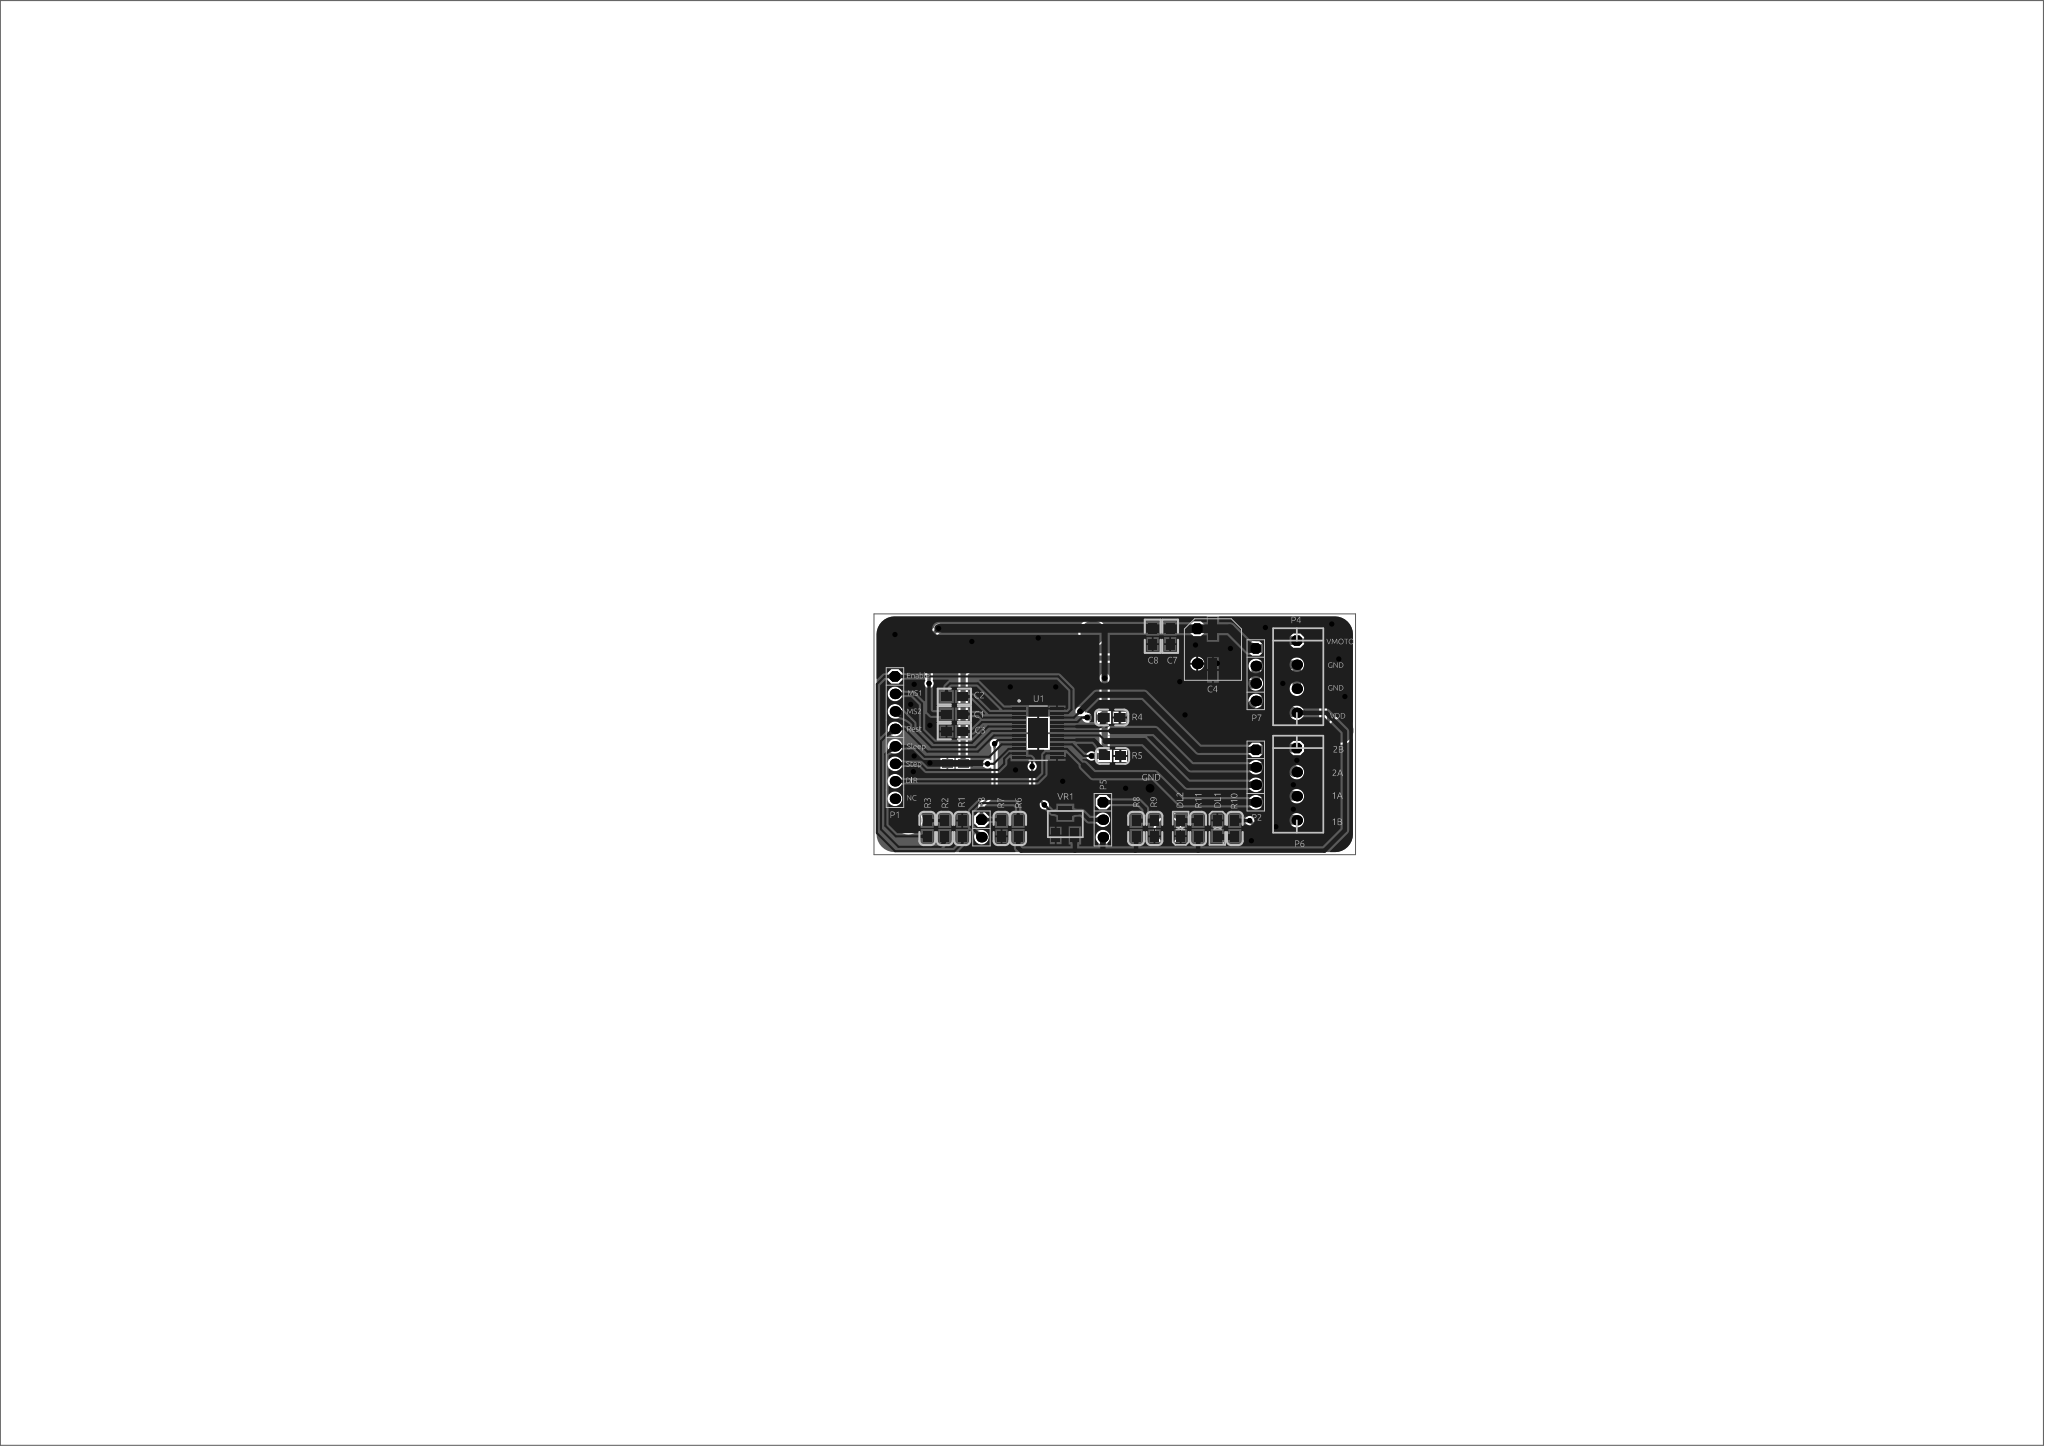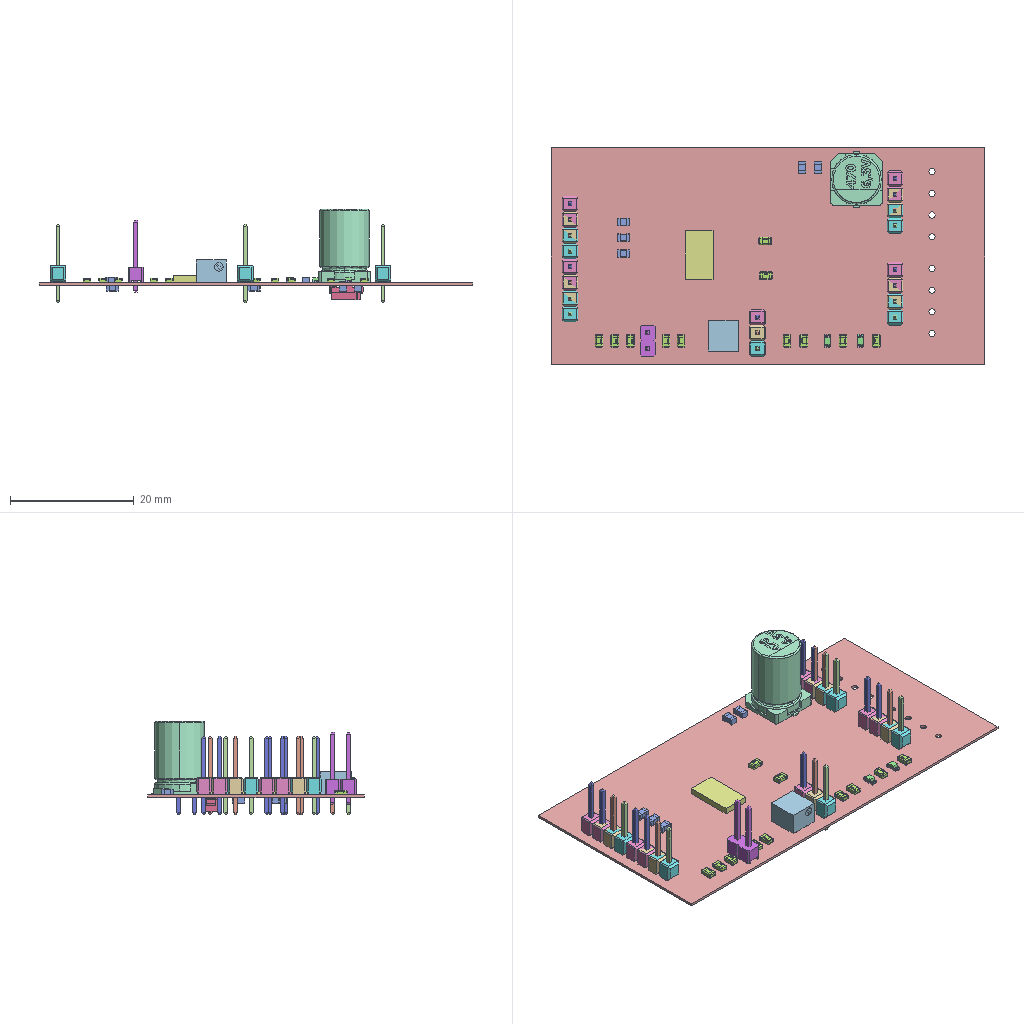Circuit board layout | Altium Designer | box 70 x 35 x 15.1 mm
Layer stack:
# Altium Designer layer stack of  (unit mm; dielectric type: 0 none, 1 core, 2 prepreg, 3 surface material)
index,name,kind,layer,copper_thickness_mm,dielectric_type,dielectric_thickness_mm,dielectric_material,dielectric_constant
0,Top Paste,other,,,,,,
1,Top Overlay,other,,,,,,
2,Top Solder,dielectric,,,3,0.0102,Solder Resist,3.5
3,Top Layer,copper,Top Layer,0.0356,,,,
4,Dielectric 1,dielectric,,,0,0.32,FR-4,4.8
5,Bottom Layer,copper,Bottom Layer,0.0356,,,,
6,Bottom Solder,dielectric,,,3,0.0102,Solder Resist,3.5
7,Bottom Overlay,other,,,,,,
8,Bottom Paste,other,,,,,,
# drill layer pairs: low layer,high layer
drill_pair,Top Layer,Bottom Layer
Part placement:
Designator,Comment,Layer,Footprint,Center-X(mm),Center-Y(mm),Rotation
C10,0.1uF,BottomLayer,0805C,34.671,19.939,360
C11,0.1uF,BottomLayer,0805C,11.811,13.208,180
R11,4.7KΩ,TopLayer,0805R,47.117,3.81,90
R10,2.5KΩ,TopLayer,0805R,52.451,3.81,270
R8,2KΩ,TopLayer,0805R,38.1,3.81,90
R7,0Ω,TopLayer,0805R,18.542,3.81,90
R6,0Ω,TopLayer,0805R,20.955,3.81,270
R5,0.47Ω,TopLayer,0805R,34.671,14.351,180
R4,0.47Ω,TopLayer,0805R,34.544,19.939,180
R3,100KΩ,TopLayer,0805R,7.747,3.81,90
R2,100KΩ,TopLayer,0805R,10.287,3.81,90
R1,10KΩ,TopLayer,0805R,12.827,3.81,90
DL2,COLOR,TopLayer,0805D,44.577,3.837,270
DL1,COLOR,TopLayer,0805D,49.911,3.837,90
C9,0.1uF,BottomLayer,0805C,34.671,14.351,360
C8,0.1uF,TopLayer,0805C,40.513,31.75,270
C7,1uF,TopLayer,0805C,43.053,31.75,270
C6,0.1uF,BottomLayer,0805C,51.435,20.32,270
C5,1uF,BottomLayer,0805C,49.022,20.32,270
C3,0.22uF,TopLayer,0805C,11.684,17.907,180
C2,0.1uF,TopLayer,0805C,11.684,22.987,180
C1,0.1uF,TopLayer,0805C,11.684,20.447,360
D1,1N5822,BottomLayer,1N5822,49.53,24.765,360
R9,3KΩ,TopLayer,0805R,40.767,3.81,270
VR1,10KΩ,TopLayer,3224W,27.813,4.445,0
U1,Value,TopLayer,A4982,23.876,17.653,0
P7,Header(4PIN),TopLayer,排针(4PIN),55.499,26.162,270
P6,VH-3.5-4PIN,TopLayer,VH-3.5-4PIN,61.468,10.244,270
P5,Pin header (3PIN),TopLayer,排针(3PIN),33.274,5.08,270
P3,Header2PIN,TopLayer,排针2PIN,15.621,3.81,270
P2,Header(4PIN),TopLayer,排针(4PIN),55.499,11.43,270
P1,Header(8PIN),TopLayer,排针（8PIN）,3.048,17.018,270
C4,470uF,TopLayer,CAP-SMD_Aluminum_Capacitors_F8_220uF_35V,49.276,29.845,270
P4,VH-3.5-4PIN,TopLayer,VH-3.5-4PIN,61.468,25.865,270
Pad and via stacks:
# Altium Designer via and pad stacks of  (unit mm). Each distinct definition once, with the count of objects using it.
# via: kind,start_layer,end_layer,hole_mm,diameter_mm,mode(0 simple;1 top-mid-bottom;2 full stack),diameter_per_layer,count,example_net
# pad: kind,layer,hole_mm,hole_type(0 round;1 square;2 slot),plating,top_size,top_shape(1 round;2 rect;3 octagon;9 rounded rect),mid_size,bottom_size,mode,footprint,size_per_layer,count,example
pad,Top Layer,0,0,plated,3.2x1.2,2,3.2x1.2,3.2x1.2,0,CAP-SMD Aluminum Capacitors F8 220uF 35V,,2,C4.2
pad,Top Layer,0,0,plated,2x2.032,2,2x2.032,2x2.032,0,3224W,,1,VR1.2
pad,Top Layer,0,0,plated,1.2x2.032,2,1.2x2.032,1.2x2.032,0,3224W,,2,VR1.1
pad,Top Layer,0,0,plated,0.4x2,2,0.4x2,0.4x2,0,A4982,,24,U1.13
pad,Top Layer,0,0,plated,2.85x4.32,2,2.85x4.32,2.85x4.32,0,A4982,,1,U1.24
pad,Top Layer,0,0,plated,1.524x1.27,2,1.524x1.27,1.524x1.27,0,0805R,,22,R9.2
pad,Top Layer,0,0,plated,1.524x1.27,2,1.524x1.27,1.524x1.27,0,0805D,,4,DL2.1
pad,Top Layer,0,0,plated,1.524x1.27,2,1.524x1.27,1.524x1.27,0,0805C,,10,C7.1
pad,Multi-Layer,0.889,0,plated,1.575x1.575,1,1.575x1.575,1.575x1.575,0,,,1,2
pad,Multi-Layer,0.889,0,plated,1.575x1.575,3,1.575x1.575,1.575x1.575,0,,,1,1
pad,Multi-Layer,1,0,plated,1.5x1.5,3,1.5x1.5,1.5x1.5,0,VH-3.5-4PIN,,2,P6.1
pad,Multi-Layer,1,0,plated,1.5x1.5,1,1.5x1.5,1.5x1.5,0,VH-3.5-4PIN,,6,P6.2
pad,Multi-Layer,0.762,0,plated,1.524x1.524,3,1.524x1.524,1.524x1.524,0,\u00C5\u00C5\u00D5\u00EB2PIN,,1,P3.1
pad,Multi-Layer,0.762,0,plated,1.524x1.524,1,1.524x1.524,1.524x1.524,0,\u00C5\u00C5\u00D5\u00EB2PIN,,1,P3.2
pad,Multi-Layer,0.762,0,plated,1.524x1.524,1,1.524x1.524,1.524x1.524,0,\u00C5\u00C5\u00D5\u00EB\u00A3\u00A88PIN\u00A3\u00A9,,7,P1.7
pad,Multi-Layer,0.762,0,plated,1.524x1.524,3,1.524x1.524,1.524x1.524,0,\u00C5\u00C5\u00D5\u00EB\u00A3\u00A88PIN\u00A3\u00A9,,1,P1.1
pad,Multi-Layer,0.762,0,plated,1.524x1.524,1,1.524x1.524,1.524x1.524,0,\u00C5\u00C5\u00D5\u00EB(3PIN),,2,P5.3
pad,Multi-Layer,0.762,0,plated,1.524x1.524,3,1.524x1.524,1.524x1.524,0,\u00C5\u00C5\u00D5\u00EB(3PIN),,1,P5.1
pad,Multi-Layer,0.9,0,plated,1.524x1.524,1,1.524x1.524,1.524x1.524,0,\u00C5\u00C5\u00D5\u00EB(4PIN),,6,P2.4
pad,Multi-Layer,0.9,0,plated,1.524x1.524,3,1.524x1.524,1.524x1.524,0,\u00C5\u00C5\u00D5\u00EB(4PIN),,2,P2.1
pad,Bottom Layer,0,0,plated,1.524x1.27,2,1.524x1.27,1.524x1.27,0,0805C,,10,C9.1
pad,Bottom Layer,0,0,plated,1.524x2.032,2,1.524x2.032,1.524x2.032,0,1N5822,,2,D1.1
pad,Bottom Layer,0,0,plated,2.85x4.32,2,2.85x4.32,2.85x4.32,0,A4982,,1,U1.24
pad,Bottom Layer,0,0,plated,3.5x3.5,1,3.5x3.5,3.5x3.5,0,,,5,0
via,Top Layer,Bottom Layer,0.381,0.762,0,,40,GND
via,Top Layer,Bottom Layer,2.032,2.54,0,,1,GND
via,Top Layer,Bottom Layer,1.016,1.27,0,,1,GND
Copper pours:
name,layer,net,type(0 solid;1 hatched;2 none)
Top Layer,Top Layer,GND,0
Top Layer,Bottom Layer,GND,0
Design rules, without the lines most boards share:
# Altium Designer design rules of  (exported by Altium Designer, unit mm)
# columns: name | kind | enabled | priority | scope1 | scope2 | descriptor | typed fields (field=value)
Clearance | 0 | enabled | 2 | All | All | Clearance Constraint (Gap=8mil) (All),(All) | gap=0.2032
PlaneConnect | 6 | enabled | 1 | All | All | Power Plane Connect Rule(Relief Connect )(Expansion=20mil) (Conductor Width=10mil) (Air Gap=10mil) (Entries=4) (All) | relief_conductor_width=0.254 relief_entries=4 relief_expansion=0.508
PolygonConnect | 20 | enabled | 2 | All | All | Polygon Connect Rule(Relief Connect )(Conductor Width=10mil) (Relief Angle=90 Angle) (Entries=4) (Air Gap Width=10mil) (All),(All) | connect_style(0=relief,1=direct,2=none)=0 relief_conductor_width=0.254 relief_entries=4
Width | 2 | enabled | 1 | All | All | Width Constraint (Min=8mil) (Max=100mil) (Preferred=20mil) (All) |
RoutingVias | 11 | enabled | 1 | All | All | Routing Via (MinHoleWidth=12mil) (MaxHoleWidth=100mil) (PreferredHoleWidth=28mil) (MinWidth=25mil) (MaxWidth=100mil) (PreferedWidth=50mil) (All) | via_min_hole=0.3048 via_max_hole=2.54 via_preferred_diameter=1.27 via_preferred_hole=0.7112
PasteMaskExpansion | 14 | enabled | 1 | All | All | Paste Mask Expansion (Expansion =0mil) (All) | expansion=0
SolderMaskExpansion | 13 | enabled | 1 | All | All | Solder Mask Expansion (Expansion =4mil) (All) | expansion=0.1016
HoleSize | 42 | enabled | 1 | All | All | Hole Size Constraint (Min=1mil) (Max=200mil) (All) |
DiffPairsRouting | 51 | enabled | 1 | All | All | Differential Pairs Uncoupled Length using the Gap Constraints (Min=10mil) (Max=10mil) (Prefered=10mil)  and Width Constraints (Min=15mil) (Max=15mil) (Prefered=15mil) (All) |
HoleToHoleClearance | 52 | enabled | 1 | All | All | Hole To Hole Clearance (Gap=5mil) (All),(All) | gap=0.127
MinimumSolderMaskSliver | 53 | enabled | 1 | All | All | Minimum Solder Mask Sliver (Gap=0mil) (All),(All) |
SilkToSolderMaskClearance | 54 | enabled | 1 | IsPad | All | Silk To Solder Mask (Clearance=0mil) (IsPad),(All) |
SilkToSilkClearance | 55 | enabled | 1 | All | All | Silk to Silk (Clearance=5mil) (All),(All) |
SilkToBoardRegionClearance | 59 | disabled | 1 | All | All | Silk primitive without silk layer |
Ploy | 0 | enabled | 1 | InPolygon | All | Clearance Constraint (Gap=12mil) (InPolygon),(All) | gap=0.3048
IsPloy | 20 | enabled | 1 | IsVia | All | Polygon Connect Rule(Direct Connect )(Conductor Width=10mil) (Relief Angle=90 Angle) (Entries=4) (Air Gap Width=10mil) (IsVia),(All) | connect_style(0=relief,1=direct,2=none)=1 relief_conductor_width=0.254 relief_entries=4
Classes set for this board:
# Altium Designer classes of  (member kind: 0 net, 1 component, 2 from-to, 3 pad, 4 layer, 5 differential pair, 6 design channel, 7 polygon, 8 structure, 9 xSignal)
# columns: class name | member kind | superclass | members
A4982 | 1 | no | C1; C2; C4; C5; C6; C7; C8; C9; C*1; DL1; DL2; R1; R2; R3; R4; R6; R*1; R*2; R*3; R*4; R*5; U1; VR1; R5; C4; R9; R9; P3; P1; P6; C4; P5; P7; D1; C1; C2; C3; C5; C6; C7; C8; C9; DL1; DL2; R1; R2; R3; R4; R5; R6; R7; R8; R10; R11; P1; C11; P2; C10; P4;